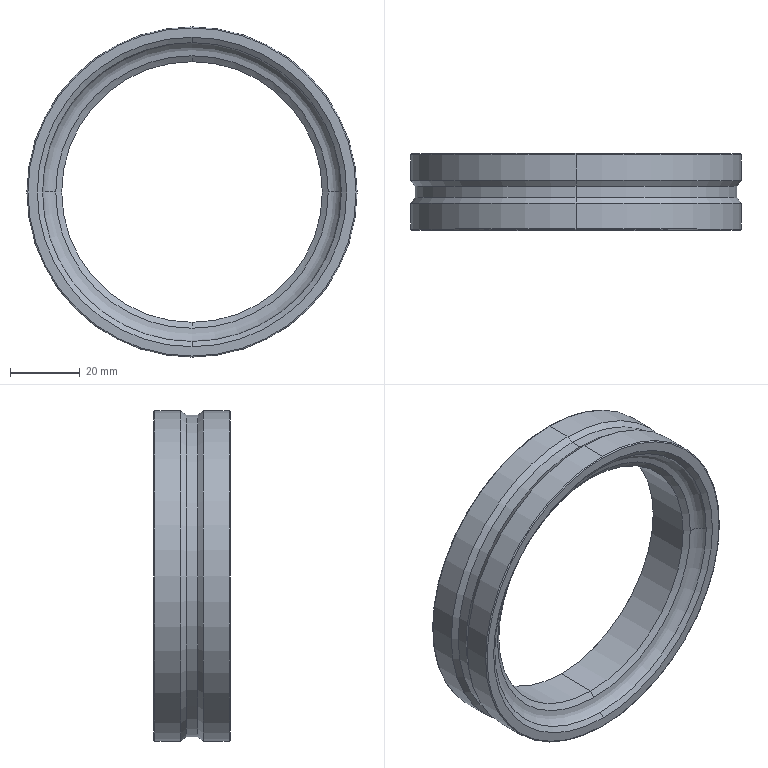Part | SolidWorks | features BaseBody 1 | 1 solid | 30 faces | box 95 x 22 x 95 mm | volume 47196 mm3 | cone 12 | torus 8 | cylinder 8 | plane 2 | commonest cylinder face diameters 95 x4 75 x2 92.6 x2
STEP:
#1=CARTESIAN_POINT('',(-2132.95,902.097,-1533.124));
#2=VERTEX_POINT('',#1);
#3=CARTESIAN_POINT('',(-2132.95,902.097,-1622.124));
#4=VERTEX_POINT('',#3);
#5=CARTESIAN_POINT('',(-2132.95,902.097,-1577.624));
#6=DIRECTION('',(0.,-1.,0.));
#7=DIRECTION('',(0.,0.,1.));
#8=AXIS2_PLACEMENT_3D('',#5,#6,#7);
#9=CIRCLE('',#8,44.5);
#10=EDGE_CURVE('',#2,#4,#9,.T.);
#11=ORIENTED_EDGE('',*,*,#10,.F.);
#12=CARTESIAN_POINT('',(-2132.95,902.097,-1577.624));
#13=DIRECTION('',(0.,-1.,0.));
#14=DIRECTION('',(0.,0.,-1.));
#15=AXIS2_PLACEMENT_3D('',#12,#13,#14);
#16=CIRCLE('',#15,44.5);
#17=EDGE_CURVE('',#4,#2,#16,.T.);
#18=ORIENTED_EDGE('',*,*,#17,.F.);
#19=EDGE_LOOP('',(#11,#18));
#20=FACE_BOUND('',#19,.T.);
#21=CARTESIAN_POINT('',(-2180.15,902.097,-1577.624));
#22=VERTEX_POINT('',#21);
#23=CARTESIAN_POINT('',(-2085.75,902.097,-1577.624));
#24=VERTEX_POINT('',#23);
#25=CARTESIAN_POINT('',(-2132.95,902.097,-1577.624));
#26=DIRECTION('',(0.,-1.,0.));
#27=DIRECTION('',(-1.,0.,0.));
#28=AXIS2_PLACEMENT_3D('',#25,#26,#27);
#29=CIRCLE('',#28,47.2);
#30=EDGE_CURVE('',#22,#24,#29,.T.);
#31=ORIENTED_EDGE('',*,*,#30,.T.);
#32=CARTESIAN_POINT('',(-2132.95,902.097,-1577.624));
#33=DIRECTION('',(0.,-1.,0.));
#34=DIRECTION('',(1.,0.,0.));
#35=AXIS2_PLACEMENT_3D('',#32,#33,#34);
#36=CIRCLE('',#35,47.2);
#37=EDGE_CURVE('',#24,#22,#36,.T.);
#38=ORIENTED_EDGE('',*,*,#37,.T.);
#39=EDGE_LOOP('',(#31,#38));
#40=FACE_OUTER_BOUND('',#39,.T.);
#41=CARTESIAN_POINT('',(-2081.03,902.097,-1629.544));
#42=DIRECTION('',(0.,-1.,0.));
#43=DIRECTION('',(0.,0.,-1.));
#44=AXIS2_PLACEMENT_3D('',#41,#42,#43);
#45=PLANE('',#44);
#46=ADVANCED_FACE('',(#20,#40),#45,.T.);
#47=CARTESIAN_POINT('',(-2132.95,903.147,-1620.624));
#48=VERTEX_POINT('',#47);
#49=CARTESIAN_POINT('',(-2132.95,902.097,-1622.124));
#50=DIRECTION('',(0.,0.5736,0.8192));
#51=VECTOR('',#50,1000.);
#52=LINE('',#49,#51);
#53=EDGE_CURVE('',#4,#48,#52,.T.);
#54=ORIENTED_EDGE('',*,*,#53,.T.);
#55=CARTESIAN_POINT('',(-2175.95,903.147,-1577.624));
#56=VERTEX_POINT('',#55);
#57=CARTESIAN_POINT('',(-2132.95,903.147,-1577.624));
#58=DIRECTION('',(0.,1.,0.));
#59=DIRECTION('',(0.,0.,-1.));
#60=AXIS2_PLACEMENT_3D('',#57,#58,#59);
#61=CIRCLE('',#60,43.);
#62=EDGE_CURVE('',#48,#56,#61,.T.);
#63=ORIENTED_EDGE('',*,*,#62,.T.);
#64=CARTESIAN_POINT('',(-2132.95,903.147,-1534.624));
#65=VERTEX_POINT('',#64);
#66=CARTESIAN_POINT('',(-2132.95,903.147,-1577.624));
#67=DIRECTION('',(0.,1.,0.));
#68=DIRECTION('',(-1.,0.,0.));
#69=AXIS2_PLACEMENT_3D('',#66,#67,#68);
#70=CIRCLE('',#69,43.);
#71=EDGE_CURVE('',#56,#65,#70,.T.);
#72=ORIENTED_EDGE('',*,*,#71,.T.);
#73=CARTESIAN_POINT('',(-2132.95,903.147,-1534.624));
#74=DIRECTION('',(0.,-0.5736,0.8192));
#75=VECTOR('',#74,1000.);
#76=LINE('',#73,#75);
#77=EDGE_CURVE('',#65,#2,#76,.T.);
#78=ORIENTED_EDGE('',*,*,#77,.T.);
#79=ORIENTED_EDGE('',*,*,#10,.T.);
#80=EDGE_LOOP('',(#54,#63,#72,#78,#79));
#81=FACE_OUTER_BOUND('',#80,.T.);
#82=CARTESIAN_POINT('',(-2132.95,903.2,-1577.624));
#83=DIRECTION('',(0.,-1.,0.));
#84=DIRECTION('',(0.08716,0.,-0.9962));
#85=AXIS2_PLACEMENT_3D('',#82,#83,#84);
#86=CONICAL_SURFACE('',#85,42.925,0.9599);
#87=ADVANCED_FACE('',(#81),#86,.F.);
#88=CARTESIAN_POINT('',(-2093.76,905.815,-1577.624));
#89=VERTEX_POINT('',#88);
#90=CARTESIAN_POINT('',(-2089.95,903.147,-1577.624));
#91=VERTEX_POINT('',#90);
#92=CARTESIAN_POINT('',(-2093.7,901.847,-1577.624));
#93=DIRECTION('',(0.,0.,-1.));
#94=DIRECTION('',(-0.01527,0.9999,0.));
#95=AXIS2_PLACEMENT_3D('',#92,#93,#94);
#96=CIRCLE('',#95,3.969);
#97=EDGE_CURVE('',#89,#91,#96,.T.);
#98=ORIENTED_EDGE('',*,*,#97,.T.);
#99=CARTESIAN_POINT('',(-2132.95,903.147,-1577.624));
#100=DIRECTION('',(0.,1.,0.));
#101=DIRECTION('',(0.,0.,1.));
#102=AXIS2_PLACEMENT_3D('',#99,#100,#101);
#103=CIRCLE('',#102,43.);
#104=EDGE_CURVE('',#65,#91,#103,.T.);
#105=ORIENTED_EDGE('',*,*,#104,.F.);
#106=ORIENTED_EDGE('',*,*,#71,.F.);
#107=CARTESIAN_POINT('',(-2172.139,905.815,-1577.624));
#108=VERTEX_POINT('',#107);
#109=CARTESIAN_POINT('',(-2172.2,901.847,-1577.624));
#110=DIRECTION('',(0.,0.,-1.));
#111=DIRECTION('',(-0.9448,0.3276,0.));
#112=AXIS2_PLACEMENT_3D('',#109,#110,#111);
#113=CIRCLE('',#112,3.969);
#114=EDGE_CURVE('',#56,#108,#113,.T.);
#115=ORIENTED_EDGE('',*,*,#114,.T.);
#116=CARTESIAN_POINT('',(-2132.95,905.815,-1538.435));
#117=VERTEX_POINT('',#116);
#118=CARTESIAN_POINT('',(-2132.95,905.815,-1577.624));
#119=DIRECTION('',(0.,1.,0.));
#120=DIRECTION('',(-1.,0.,0.));
#121=AXIS2_PLACEMENT_3D('',#118,#119,#120);
#122=CIRCLE('',#121,39.189);
#123=EDGE_CURVE('',#108,#117,#122,.T.);
#124=ORIENTED_EDGE('',*,*,#123,.T.);
#125=CARTESIAN_POINT('',(-2132.95,905.815,-1577.624));
#126=DIRECTION('',(0.,1.,0.));
#127=DIRECTION('',(0.,0.,1.));
#128=AXIS2_PLACEMENT_3D('',#125,#126,#127);
#129=CIRCLE('',#128,39.189);
#130=EDGE_CURVE('',#117,#89,#129,.T.);
#131=ORIENTED_EDGE('',*,*,#130,.T.);
#132=EDGE_LOOP('',(#98,#105,#106,#115,#124,#131));
#133=FACE_OUTER_BOUND('',#132,.T.);
#134=CARTESIAN_POINT('',(-2132.95,901.847,-1577.624));
#135=DIRECTION('',(0.,1.,0.));
#136=DIRECTION('',(-0.9962,0.,-0.08716));
#137=AXIS2_PLACEMENT_3D('',#134,#135,#136);
#138=TOROIDAL_SURFACE('',#137,39.25,3.969);
#139=ADVANCED_FACE('',(#133),#138,.F.);
#140=CARTESIAN_POINT('',(-2132.95,905.815,-1616.814));
#141=VERTEX_POINT('',#140);
#142=CARTESIAN_POINT('',(-2132.95,906.998,-1615.124));
#143=VERTEX_POINT('',#142);
#144=CARTESIAN_POINT('',(-2132.95,905.815,-1616.814));
#145=DIRECTION('',(0.,0.5736,0.8192));
#146=VECTOR('',#145,1000.);
#147=LINE('',#144,#146);
#148=EDGE_CURVE('',#141,#143,#147,.T.);
#149=ORIENTED_EDGE('',*,*,#148,.T.);
#150=CARTESIAN_POINT('',(-2132.95,906.998,-1540.124));
#151=VERTEX_POINT('',#150);
#152=CARTESIAN_POINT('',(-2132.95,906.998,-1577.624));
#153=DIRECTION('',(0.,1.,0.));
#154=DIRECTION('',(0.,0.,-1.));
#155=AXIS2_PLACEMENT_3D('',#152,#153,#154);
#156=CIRCLE('',#155,37.5);
#157=EDGE_CURVE('',#143,#151,#156,.T.);
#158=ORIENTED_EDGE('',*,*,#157,.T.);
#159=CARTESIAN_POINT('',(-2132.95,906.998,-1540.124));
#160=DIRECTION('',(0.,-0.5736,0.8192));
#161=VECTOR('',#160,1000.);
#162=LINE('',#159,#161);
#163=EDGE_CURVE('',#151,#117,#162,.T.);
#164=ORIENTED_EDGE('',*,*,#163,.T.);
#165=ORIENTED_EDGE('',*,*,#123,.F.);
#166=CARTESIAN_POINT('',(-2132.95,905.815,-1577.624));
#167=DIRECTION('',(0.,1.,0.));
#168=DIRECTION('',(0.,0.,-1.));
#169=AXIS2_PLACEMENT_3D('',#166,#167,#168);
#170=CIRCLE('',#169,39.189);
#171=EDGE_CURVE('',#141,#108,#170,.T.);
#172=ORIENTED_EDGE('',*,*,#171,.F.);
#173=EDGE_LOOP('',(#149,#158,#164,#165,#172));
#174=FACE_OUTER_BOUND('',#173,.T.);
#175=CARTESIAN_POINT('',(-2132.95,907.057,-1577.624));
#176=DIRECTION('',(0.,-1.,0.));
#177=DIRECTION('',(0.08716,0.,-0.9962));
#178=AXIS2_PLACEMENT_3D('',#175,#176,#177);
#179=CONICAL_SURFACE('',#178,37.416,0.9599);
#180=ADVANCED_FACE('',(#174),#179,.F.);
#181=CARTESIAN_POINT('',(-2132.95,919.195,-1615.124));
#182=VERTEX_POINT('',#181);
#183=CARTESIAN_POINT('',(-2132.95,906.998,-1615.124));
#184=DIRECTION('',(0.,1.,0.));
#185=VECTOR('',#184,1000.);
#186=LINE('',#183,#185);
#187=EDGE_CURVE('',#143,#182,#186,.T.);
#188=ORIENTED_EDGE('',*,*,#187,.T.);
#189=CARTESIAN_POINT('',(-2132.95,919.195,-1540.124));
#190=VERTEX_POINT('',#189);
#191=CARTESIAN_POINT('',(-2132.95,919.195,-1577.624));
#192=DIRECTION('',(0.,1.,0.));
#193=DIRECTION('',(0.,0.,-1.));
#194=AXIS2_PLACEMENT_3D('',#191,#192,#193);
#195=CIRCLE('',#194,37.5);
#196=EDGE_CURVE('',#182,#190,#195,.T.);
#197=ORIENTED_EDGE('',*,*,#196,.T.);
#198=CARTESIAN_POINT('',(-2132.95,919.195,-1540.124));
#199=DIRECTION('',(0.,-1.,0.));
#200=VECTOR('',#199,1000.);
#201=LINE('',#198,#200);
#202=EDGE_CURVE('',#190,#151,#201,.T.);
#203=ORIENTED_EDGE('',*,*,#202,.T.);
#204=ORIENTED_EDGE('',*,*,#157,.F.);
#205=EDGE_LOOP('',(#188,#197,#203,#204));
#206=FACE_OUTER_BOUND('',#205,.T.);
#207=CARTESIAN_POINT('',(-2132.95,919.805,-1577.624));
#208=DIRECTION('',(0.,-1.,0.));
#209=DIRECTION('',(0.08716,0.,0.9962));
#210=AXIS2_PLACEMENT_3D('',#207,#208,#209);
#211=CYLINDRICAL_SURFACE('',#210,37.5);
#212=ADVANCED_FACE('',(#206),#211,.F.);
#213=CARTESIAN_POINT('',(-2132.95,920.378,-1616.814));
#214=VERTEX_POINT('',#213);
#215=CARTESIAN_POINT('',(-2132.95,919.195,-1615.124));
#216=DIRECTION('',(0.,0.5736,-0.8192));
#217=VECTOR('',#216,1000.);
#218=LINE('',#215,#217);
#219=EDGE_CURVE('',#182,#214,#218,.T.);
#220=ORIENTED_EDGE('',*,*,#219,.T.);
#221=CARTESIAN_POINT('',(-2172.139,920.378,-1577.624));
#222=VERTEX_POINT('',#221);
#223=CARTESIAN_POINT('',(-2132.95,920.378,-1577.624));
#224=DIRECTION('',(0.,1.,0.));
#225=DIRECTION('',(0.,0.,-1.));
#226=AXIS2_PLACEMENT_3D('',#223,#224,#225);
#227=CIRCLE('',#226,39.189);
#228=EDGE_CURVE('',#214,#222,#227,.T.);
#229=ORIENTED_EDGE('',*,*,#228,.T.);
#230=CARTESIAN_POINT('',(-2132.95,920.378,-1538.435));
#231=VERTEX_POINT('',#230);
#232=CARTESIAN_POINT('',(-2132.95,920.378,-1577.624));
#233=DIRECTION('',(0.,1.,0.));
#234=DIRECTION('',(-1.,0.,0.));
#235=AXIS2_PLACEMENT_3D('',#232,#233,#234);
#236=CIRCLE('',#235,39.189);
#237=EDGE_CURVE('',#222,#231,#236,.T.);
#238=ORIENTED_EDGE('',*,*,#237,.T.);
#239=CARTESIAN_POINT('',(-2132.95,920.378,-1538.435));
#240=DIRECTION('',(0.,-0.5736,-0.8192));
#241=VECTOR('',#240,1000.);
#242=LINE('',#239,#241);
#243=EDGE_CURVE('',#231,#190,#242,.T.);
#244=ORIENTED_EDGE('',*,*,#243,.T.);
#245=ORIENTED_EDGE('',*,*,#196,.F.);
#246=EDGE_LOOP('',(#220,#229,#238,#244,#245));
#247=FACE_OUTER_BOUND('',#246,.T.);
#248=CARTESIAN_POINT('',(-2132.95,919.136,-1577.624));
#249=DIRECTION('',(0.,1.,0.));
#250=DIRECTION('',(0.08716,0.,0.9962));
#251=AXIS2_PLACEMENT_3D('',#248,#249,#250);
#252=CONICAL_SURFACE('',#251,37.416,0.9599);
#253=ADVANCED_FACE('',(#247),#252,.F.);
#254=CARTESIAN_POINT('',(-2089.95,923.046,-1577.624));
#255=VERTEX_POINT('',#254);
#256=CARTESIAN_POINT('',(-2093.76,920.378,-1577.624));
#257=VERTEX_POINT('',#256);
#258=CARTESIAN_POINT('',(-2093.7,924.347,-1577.624));
#259=DIRECTION('',(0.,0.,-1.));
#260=DIRECTION('',(0.9448,-0.3276,0.));
#261=AXIS2_PLACEMENT_3D('',#258,#259,#260);
#262=CIRCLE('',#261,3.969);
#263=EDGE_CURVE('',#255,#257,#262,.T.);
#264=ORIENTED_EDGE('',*,*,#263,.T.);
#265=CARTESIAN_POINT('',(-2132.95,920.378,-1577.624));
#266=DIRECTION('',(0.,1.,0.));
#267=DIRECTION('',(0.,0.,1.));
#268=AXIS2_PLACEMENT_3D('',#265,#266,#267);
#269=CIRCLE('',#268,39.189);
#270=EDGE_CURVE('',#231,#257,#269,.T.);
#271=ORIENTED_EDGE('',*,*,#270,.F.);
#272=ORIENTED_EDGE('',*,*,#237,.F.);
#273=CARTESIAN_POINT('',(-2175.95,923.046,-1577.624));
#274=VERTEX_POINT('',#273);
#275=CARTESIAN_POINT('',(-2172.2,924.347,-1577.624));
#276=DIRECTION('',(0.,0.,-1.));
#277=DIRECTION('',(0.01527,-0.9999,0.));
#278=AXIS2_PLACEMENT_3D('',#275,#276,#277);
#279=CIRCLE('',#278,3.969);
#280=EDGE_CURVE('',#222,#274,#279,.T.);
#281=ORIENTED_EDGE('',*,*,#280,.T.);
#282=CARTESIAN_POINT('',(-2132.95,923.046,-1534.624));
#283=VERTEX_POINT('',#282);
#284=CARTESIAN_POINT('',(-2132.95,923.046,-1577.624));
#285=DIRECTION('',(0.,1.,0.));
#286=DIRECTION('',(-1.,0.,0.));
#287=AXIS2_PLACEMENT_3D('',#284,#285,#286);
#288=CIRCLE('',#287,43.);
#289=EDGE_CURVE('',#274,#283,#288,.T.);
#290=ORIENTED_EDGE('',*,*,#289,.T.);
#291=CARTESIAN_POINT('',(-2132.95,923.046,-1577.624));
#292=DIRECTION('',(0.,1.,0.));
#293=DIRECTION('',(0.,0.,1.));
#294=AXIS2_PLACEMENT_3D('',#291,#292,#293);
#295=CIRCLE('',#294,43.);
#296=EDGE_CURVE('',#283,#255,#295,.T.);
#297=ORIENTED_EDGE('',*,*,#296,.T.);
#298=EDGE_LOOP('',(#264,#271,#272,#281,#290,#297));
#299=FACE_OUTER_BOUND('',#298,.T.);
#300=CARTESIAN_POINT('',(-2132.95,924.347,-1577.624));
#301=DIRECTION('',(0.,1.,0.));
#302=DIRECTION('',(-0.9962,0.,-0.08716));
#303=AXIS2_PLACEMENT_3D('',#300,#301,#302);
#304=TOROIDAL_SURFACE('',#303,39.25,3.969);
#305=ADVANCED_FACE('',(#299),#304,.F.);
#306=CARTESIAN_POINT('',(-2132.95,923.046,-1620.624));
#307=VERTEX_POINT('',#306);
#308=CARTESIAN_POINT('',(-2132.95,924.097,-1622.124));
#309=VERTEX_POINT('',#308);
#310=CARTESIAN_POINT('',(-2132.95,923.046,-1620.624));
#311=DIRECTION('',(0.,0.5736,-0.8192));
#312=VECTOR('',#311,1000.);
#313=LINE('',#310,#312);
#314=EDGE_CURVE('',#307,#309,#313,.T.);
#315=ORIENTED_EDGE('',*,*,#314,.T.);
#316=CARTESIAN_POINT('',(-2132.95,924.097,-1533.124));
#317=VERTEX_POINT('',#316);
#318=CARTESIAN_POINT('',(-2132.95,924.097,-1577.624));
#319=DIRECTION('',(0.,1.,0.));
#320=DIRECTION('',(0.,0.,-1.));
#321=AXIS2_PLACEMENT_3D('',#318,#319,#320);
#322=CIRCLE('',#321,44.5);
#323=EDGE_CURVE('',#309,#317,#322,.T.);
#324=ORIENTED_EDGE('',*,*,#323,.T.);
#325=CARTESIAN_POINT('',(-2132.95,924.097,-1533.124));
#326=DIRECTION('',(0.,-0.5736,-0.8192));
#327=VECTOR('',#326,1000.);
#328=LINE('',#325,#327);
#329=EDGE_CURVE('',#317,#283,#328,.T.);
#330=ORIENTED_EDGE('',*,*,#329,.T.);
#331=ORIENTED_EDGE('',*,*,#289,.F.);
#332=CARTESIAN_POINT('',(-2132.95,923.046,-1577.624));
#333=DIRECTION('',(0.,1.,0.));
#334=DIRECTION('',(0.,0.,-1.));
#335=AXIS2_PLACEMENT_3D('',#332,#333,#334);
#336=CIRCLE('',#335,43.);
#337=EDGE_CURVE('',#307,#274,#336,.T.);
#338=ORIENTED_EDGE('',*,*,#337,.F.);
#339=EDGE_LOOP('',(#315,#324,#330,#331,#338));
#340=FACE_OUTER_BOUND('',#339,.T.);
#341=CARTESIAN_POINT('',(-2132.95,922.994,-1577.624));
#342=DIRECTION('',(0.,1.,0.));
#343=DIRECTION('',(0.08716,0.,0.9962));
#344=AXIS2_PLACEMENT_3D('',#341,#342,#343);
#345=CONICAL_SURFACE('',#344,42.925,0.9599);
#346=ADVANCED_FACE('',(#340),#345,.F.);
#347=ORIENTED_EDGE('',*,*,#323,.F.);
#348=CARTESIAN_POINT('',(-2132.95,924.097,-1577.624));
#349=DIRECTION('',(0.,1.,0.));
#350=DIRECTION('',(0.,0.,1.));
#351=AXIS2_PLACEMENT_3D('',#348,#349,#350);
#352=CIRCLE('',#351,44.5);
#353=EDGE_CURVE('',#317,#309,#352,.T.);
#354=ORIENTED_EDGE('',*,*,#353,.F.);
#355=EDGE_LOOP('',(#347,#354));
#356=FACE_BOUND('',#355,.T.);
#357=CARTESIAN_POINT('',(-2085.75,924.097,-1577.624));
#358=VERTEX_POINT('',#357);
#359=CARTESIAN_POINT('',(-2180.15,924.097,-1577.624));
#360=VERTEX_POINT('',#359);
#361=CARTESIAN_POINT('',(-2132.95,924.097,-1577.624));
#362=DIRECTION('',(0.,1.,0.));
#363=DIRECTION('',(0.,0.,-1.));
#364=AXIS2_PLACEMENT_3D('',#361,#362,#363);
#365=CIRCLE('',#364,47.2);
#366=EDGE_CURVE('',#358,#360,#365,.T.);
#367=ORIENTED_EDGE('',*,*,#366,.T.);
#368=CARTESIAN_POINT('',(-2132.95,924.097,-1577.624));
#369=DIRECTION('',(0.,1.,0.));
#370=DIRECTION('',(-1.,0.,0.));
#371=AXIS2_PLACEMENT_3D('',#368,#369,#370);
#372=CIRCLE('',#371,47.2);
#373=EDGE_CURVE('',#360,#358,#372,.T.);
#374=ORIENTED_EDGE('',*,*,#373,.T.);
#375=EDGE_LOOP('',(#367,#374));
#376=FACE_OUTER_BOUND('',#375,.T.);
#377=CARTESIAN_POINT('',(-2081.03,924.097,-1525.704));
#378=DIRECTION('',(0.,1.,0.));
#379=DIRECTION('',(1.,0.,0.));
#380=AXIS2_PLACEMENT_3D('',#377,#378,#379);
#381=PLANE('',#380);
#382=ADVANCED_FACE('',(#356,#376),#381,.T.);
#383=CARTESIAN_POINT('',(-2180.45,923.797,-1577.624));
#384=VERTEX_POINT('',#383);
#385=CARTESIAN_POINT('',(-2180.15,923.797,-1577.624));
#386=DIRECTION('',(0.,0.,-1.));
#387=DIRECTION('',(-1.,0.,0.));
#388=AXIS2_PLACEMENT_3D('',#385,#386,#387);
#389=CIRCLE('',#388,0.3);
#390=EDGE_CURVE('',#384,#360,#389,.T.);
#391=ORIENTED_EDGE('',*,*,#390,.T.);
#392=ORIENTED_EDGE('',*,*,#366,.F.);
#393=CARTESIAN_POINT('',(-2085.45,923.797,-1577.624));
#394=VERTEX_POINT('',#393);
#395=CARTESIAN_POINT('',(-2085.75,923.797,-1577.624));
#396=DIRECTION('',(0.,0.,-1.));
#397=DIRECTION('',(0.,1.,0.));
#398=AXIS2_PLACEMENT_3D('',#395,#396,#397);
#399=CIRCLE('',#398,0.3);
#400=EDGE_CURVE('',#358,#394,#399,.T.);
#401=ORIENTED_EDGE('',*,*,#400,.T.);
#402=CARTESIAN_POINT('',(-2132.95,923.797,-1625.124));
#403=VERTEX_POINT('',#402);
#404=CARTESIAN_POINT('',(-2132.95,923.797,-1577.624));
#405=DIRECTION('',(0.,1.,0.));
#406=DIRECTION('',(1.,0.,0.));
#407=AXIS2_PLACEMENT_3D('',#404,#405,#406);
#408=CIRCLE('',#407,47.5);
#409=EDGE_CURVE('',#394,#403,#408,.T.);
#410=ORIENTED_EDGE('',*,*,#409,.T.);
#411=CARTESIAN_POINT('',(-2132.95,923.797,-1577.624));
#412=DIRECTION('',(0.,1.,0.));
#413=DIRECTION('',(0.,0.,-1.));
#414=AXIS2_PLACEMENT_3D('',#411,#412,#413);
#415=CIRCLE('',#414,47.5);
#416=EDGE_CURVE('',#403,#384,#415,.T.);
#417=ORIENTED_EDGE('',*,*,#416,.T.);
#418=EDGE_LOOP('',(#391,#392,#401,#410,#417));
#419=FACE_OUTER_BOUND('',#418,.T.);
#420=CARTESIAN_POINT('',(-2132.95,923.797,-1577.624));
#421=DIRECTION('',(0.,1.,0.));
#422=DIRECTION('',(0.9962,0.,0.08716));
#423=AXIS2_PLACEMENT_3D('',#420,#421,#422);
#424=TOROIDAL_SURFACE('',#423,47.2,0.3);
#425=ADVANCED_FACE('',(#419),#424,.T.);
#426=CARTESIAN_POINT('',(-2132.95,916.347,-1625.124));
#427=VERTEX_POINT('',#426);
#428=CARTESIAN_POINT('',(-2132.95,916.347,-1625.124));
#429=DIRECTION('',(0.,1.,0.));
#430=VECTOR('',#429,1000.);
#431=LINE('',#428,#430);
#432=EDGE_CURVE('',#427,#403,#431,.T.);
#433=ORIENTED_EDGE('',*,*,#432,.T.);
#434=ORIENTED_EDGE('',*,*,#409,.F.);
#435=CARTESIAN_POINT('',(-2132.95,923.797,-1530.124));
#436=VERTEX_POINT('',#435);
#437=CARTESIAN_POINT('',(-2132.95,923.797,-1577.624));
#438=DIRECTION('',(0.,1.,0.));
#439=DIRECTION('',(0.,0.,1.));
#440=AXIS2_PLACEMENT_3D('',#437,#438,#439);
#441=CIRCLE('',#440,47.5);
#442=EDGE_CURVE('',#436,#394,#441,.T.);
#443=ORIENTED_EDGE('',*,*,#442,.F.);
#444=CARTESIAN_POINT('',(-2132.95,916.347,-1530.124));
#445=VERTEX_POINT('',#444);
#446=CARTESIAN_POINT('',(-2132.95,923.797,-1530.124));
#447=DIRECTION('',(0.,-1.,0.));
#448=VECTOR('',#447,1000.);
#449=LINE('',#446,#448);
#450=EDGE_CURVE('',#436,#445,#449,.T.);
#451=ORIENTED_EDGE('',*,*,#450,.T.);
#452=CARTESIAN_POINT('',(-2132.95,916.347,-1577.624));
#453=DIRECTION('',(0.,1.,0.));
#454=DIRECTION('',(0.,0.,1.));
#455=AXIS2_PLACEMENT_3D('',#452,#453,#454);
#456=CIRCLE('',#455,47.5);
#457=EDGE_CURVE('',#445,#427,#456,.T.);
#458=ORIENTED_EDGE('',*,*,#457,.T.);
#459=EDGE_LOOP('',(#433,#434,#443,#451,#458));
#460=FACE_OUTER_BOUND('',#459,.T.);
#461=CARTESIAN_POINT('',(-2132.95,915.974,-1577.624));
#462=DIRECTION('',(0.,-1.,0.));
#463=DIRECTION('',(-0.08716,0.,-0.9962));
#464=AXIS2_PLACEMENT_3D('',#461,#462,#463);
#465=CYLINDRICAL_SURFACE('',#464,47.5);
#466=ADVANCED_FACE('',(#460),#465,.T.);
#467=CARTESIAN_POINT('',(-2132.95,914.697,-1623.924));
#468=VERTEX_POINT('',#467);
#469=CARTESIAN_POINT('',(-2132.95,914.697,-1623.924));
#470=DIRECTION('',(0.,0.8087,-0.5882));
#471=VECTOR('',#470,1000.);
#472=LINE('',#469,#471);
#473=EDGE_CURVE('',#468,#427,#472,.T.);
#474=ORIENTED_EDGE('',*,*,#473,.T.);
#475=ORIENTED_EDGE('',*,*,#457,.F.);
#476=CARTESIAN_POINT('',(-2132.95,914.697,-1531.324));
#477=VERTEX_POINT('',#476);
#478=CARTESIAN_POINT('',(-2132.95,916.347,-1530.124));
#479=DIRECTION('',(0.,-0.8087,-0.5882));
#480=VECTOR('',#479,1000.);
#481=LINE('',#478,#480);
#482=EDGE_CURVE('',#445,#477,#481,.T.);
#483=ORIENTED_EDGE('',*,*,#482,.T.);
#484=CARTESIAN_POINT('',(-2132.95,914.697,-1577.624));
#485=DIRECTION('',(0.,1.,0.));
#486=DIRECTION('',(0.,0.,1.));
#487=AXIS2_PLACEMENT_3D('',#484,#485,#486);
#488=CIRCLE('',#487,46.3);
#489=EDGE_CURVE('',#477,#468,#488,.T.);
#490=ORIENTED_EDGE('',*,*,#489,.T.);
#491=EDGE_LOOP('',(#474,#475,#483,#490));
#492=FACE_OUTER_BOUND('',#491,.T.);
#493=CARTESIAN_POINT('',(-2132.95,914.614,-1577.624));
#494=DIRECTION('',(0.,1.,0.));
#495=DIRECTION('',(-0.08716,0.,0.9962));
#496=AXIS2_PLACEMENT_3D('',#493,#494,#495);
#497=CONICAL_SURFACE('',#496,46.24,0.6288);
#498=ADVANCED_FACE('',(#492),#497,.T.);
#499=CARTESIAN_POINT('',(-2132.95,911.497,-1623.924));
#500=VERTEX_POINT('',#499);
#501=CARTESIAN_POINT('',(-2132.95,911.497,-1623.924));
#502=DIRECTION('',(0.,1.,0.));
#503=VECTOR('',#502,1000.);
#504=LINE('',#501,#503);
#505=EDGE_CURVE('',#500,#468,#504,.T.);
#506=ORIENTED_EDGE('',*,*,#505,.T.);
#507=ORIENTED_EDGE('',*,*,#489,.F.);
#508=CARTESIAN_POINT('',(-2132.95,911.497,-1531.324));
#509=VERTEX_POINT('',#508);
#510=CARTESIAN_POINT('',(-2132.95,914.697,-1531.324));
#511=DIRECTION('',(0.,-1.,0.));
#512=VECTOR('',#511,1000.);
#513=LINE('',#510,#512);
#514=EDGE_CURVE('',#477,#509,#513,.T.);
#515=ORIENTED_EDGE('',*,*,#514,.T.);
#516=CARTESIAN_POINT('',(-2132.95,911.497,-1577.624));
#517=DIRECTION('',(0.,1.,0.));
#518=DIRECTION('',(0.,0.,1.));
#519=AXIS2_PLACEMENT_3D('',#516,#517,#518);
#520=CIRCLE('',#519,46.3);
#521=EDGE_CURVE('',#509,#500,#520,.T.);
#522=ORIENTED_EDGE('',*,*,#521,.T.);
#523=EDGE_LOOP('',(#506,#507,#515,#522));
#524=FACE_OUTER_BOUND('',#523,.T.);
#525=CARTESIAN_POINT('',(-2132.95,911.337,-1577.624));
#526=DIRECTION('',(0.,-1.,0.));
#527=DIRECTION('',(-0.08716,0.,-0.9962));
#528=AXIS2_PLACEMENT_3D('',#525,#526,#527);
#529=CYLINDRICAL_SURFACE('',#528,46.3);
#530=ADVANCED_FACE('',(#524),#529,.T.);
#531=CARTESIAN_POINT('',(-2132.95,909.847,-1625.124));
#532=VERTEX_POINT('',#531);
#533=CARTESIAN_POINT('',(-2132.95,909.847,-1625.124));
#534=DIRECTION('',(0.,0.8087,0.5882));
#535=VECTOR('',#534,1000.);
#536=LINE('',#533,#535);
#537=EDGE_CURVE('',#532,#500,#536,.T.);
#538=ORIENTED_EDGE('',*,*,#537,.T.);
#539=ORIENTED_EDGE('',*,*,#521,.F.);
#540=CARTESIAN_POINT('',(-2132.95,909.847,-1530.124));
#541=VERTEX_POINT('',#540);
#542=CARTESIAN_POINT('',(-2132.95,911.497,-1531.324));
#543=DIRECTION('',(0.,-0.8087,0.5882));
#544=VECTOR('',#543,1000.);
#545=LINE('',#542,#544);
#546=EDGE_CURVE('',#509,#541,#545,.T.);
#547=ORIENTED_EDGE('',*,*,#546,.T.);
#548=CARTESIAN_POINT('',(-2132.95,909.847,-1577.624));
#549=DIRECTION('',(0.,1.,0.));
#550=DIRECTION('',(0.,0.,1.));
#551=AXIS2_PLACEMENT_3D('',#548,#549,#550);
#552=CIRCLE('',#551,47.5);
#553=EDGE_CURVE('',#541,#532,#552,.T.);
#554=ORIENTED_EDGE('',*,*,#553,.T.);
#555=EDGE_LOOP('',(#538,#539,#547,#554));
#556=FACE_OUTER_BOUND('',#555,.T.);
#557=CARTESIAN_POINT('',(-2132.95,911.579,-1577.624));
#558=DIRECTION('',(0.,-1.,0.));
#559=DIRECTION('',(-0.08716,0.,-0.9962));
#560=AXIS2_PLACEMENT_3D('',#557,#558,#559);
#561=CONICAL_SURFACE('',#560,46.24,0.6288);
#562=ADVANCED_FACE('',(#556),#561,.T.);
#563=CARTESIAN_POINT('',(-2132.95,902.397,-1625.124));
#564=VERTEX_POINT('',#563);
#565=CARTESIAN_POINT('',(-2132.95,902.397,-1625.124));
#566=DIRECTION('',(0.,1.,0.));
#567=VECTOR('',#566,1000.);
#568=LINE('',#565,#567);
#569=EDGE_CURVE('',#564,#532,#568,.T.);
#570=ORIENTED_EDGE('',*,*,#569,.T.);
#571=ORIENTED_EDGE('',*,*,#553,.F.);
#572=CARTESIAN_POINT('',(-2132.95,902.397,-1530.124));
#573=VERTEX_POINT('',#572);
#574=CARTESIAN_POINT('',(-2132.95,909.847,-1530.124));
#575=DIRECTION('',(0.,-1.,0.));
#576=VECTOR('',#575,1000.);
#577=LINE('',#574,#576);
#578=EDGE_CURVE('',#541,#573,#577,.T.);
#579=ORIENTED_EDGE('',*,*,#578,.T.);
#580=CARTESIAN_POINT('',(-2085.45,902.397,-1577.624));
#581=VERTEX_POINT('',#580);
#582=CARTESIAN_POINT('',(-2132.95,902.397,-1577.624));
#583=DIRECTION('',(0.,1.,0.));
#584=DIRECTION('',(0.,0.,1.));
#585=AXIS2_PLACEMENT_3D('',#582,#583,#584);
#586=CIRCLE('',#585,47.5);
#587=EDGE_CURVE('',#573,#581,#586,.T.);
#588=ORIENTED_EDGE('',*,*,#587,.T.);
#589=CARTESIAN_POINT('',(-2132.95,902.397,-1577.624));
#590=DIRECTION('',(0.,1.,0.));
#591=DIRECTION('',(1.,0.,0.));
#592=AXIS2_PLACEMENT_3D('',#589,#590,#591);
#593=CIRCLE('',#592,47.5);
#594=EDGE_CURVE('',#581,#564,#593,.T.);
#595=ORIENTED_EDGE('',*,*,#594,.T.);
#596=EDGE_LOOP('',(#570,#571,#579,#588,#595));
#597=FACE_OUTER_BOUND('',#596,.T.);
#598=CARTESIAN_POINT('',(-2132.95,902.024,-1577.624));
#599=DIRECTION('',(0.,-1.,0.));
#600=DIRECTION('',(-0.08716,0.,-0.9962));
#601=AXIS2_PLACEMENT_3D('',#598,#599,#600);
#602=CYLINDRICAL_SURFACE('',#601,47.5);
#603=ADVANCED_FACE('',(#597),#602,.T.);
#604=CARTESIAN_POINT('',(-2180.45,902.397,-1577.624));
#605=VERTEX_POINT('',#604);
#606=CARTESIAN_POINT('',(-2180.15,902.397,-1577.624));
#607=DIRECTION('',(0.,0.,-1.));
#608=DIRECTION('',(0.,-1.,0.));
#609=AXIS2_PLACEMENT_3D('',#606,#607,#608);
#610=CIRCLE('',#609,0.3);
#611=EDGE_CURVE('',#22,#605,#610,.T.);
#612=ORIENTED_EDGE('',*,*,#611,.T.);
#613=CARTESIAN_POINT('',(-2132.95,902.397,-1577.624));
#614=DIRECTION('',(0.,1.,0.));
#615=DIRECTION('',(0.,0.,-1.));
#616=AXIS2_PLACEMENT_3D('',#613,#614,#615);
#617=CIRCLE('',#616,47.5);
#618=EDGE_CURVE('',#564,#605,#617,.T.);
#619=ORIENTED_EDGE('',*,*,#618,.F.);
#620=ORIENTED_EDGE('',*,*,#594,.F.);
#621=CARTESIAN_POINT('',(-2085.75,902.397,-1577.624));
#622=DIRECTION('',(0.,0.,-1.));
#623=DIRECTION('',(1.,0.,0.));
#624=AXIS2_PLACEMENT_3D('',#621,#622,#623);
#625=CIRCLE('',#624,0.3);
#626=EDGE_CURVE('',#581,#24,#625,.T.);
#627=ORIENTED_EDGE('',*,*,#626,.T.);
#628=ORIENTED_EDGE('',*,*,#30,.F.);
#629=EDGE_LOOP('',(#612,#619,#620,#627,#628));
#630=FACE_OUTER_BOUND('',#629,.T.);
#631=CARTESIAN_POINT('',(-2132.95,902.397,-1577.624));
#632=DIRECTION('',(0.,1.,0.));
#633=DIRECTION('',(0.9962,0.,0.08716));
#634=AXIS2_PLACEMENT_3D('',#631,#632,#633);
#635=TOROIDAL_SURFACE('',#634,47.2,0.3);
#636=ADVANCED_FACE('',(#630),#635,.T.);
#637=ORIENTED_EDGE('',*,*,#611,.F.);
#638=ORIENTED_EDGE('',*,*,#37,.F.);
#639=ORIENTED_EDGE('',*,*,#626,.F.);
#640=ORIENTED_EDGE('',*,*,#587,.F.);
#641=CARTESIAN_POINT('',(-2132.95,902.397,-1577.624));
#642=DIRECTION('',(0.,1.,0.));
#643=DIRECTION('',(-1.,0.,0.));
#644=AXIS2_PLACEMENT_3D('',#641,#642,#643);
#645=CIRCLE('',#644,47.5);
#646=EDGE_CURVE('',#605,#573,#645,.T.);
#647=ORIENTED_EDGE('',*,*,#646,.F.);
#648=EDGE_LOOP('',(#637,#638,#639,#640,#647));
#649=FACE_OUTER_BOUND('',#648,.T.);
#650=CARTESIAN_POINT('',(-2132.95,902.397,-1577.624));
#651=DIRECTION('',(0.,1.,0.));
#652=DIRECTION('',(-0.9962,0.,-0.08716));
#653=AXIS2_PLACEMENT_3D('',#650,#651,#652);
#654=TOROIDAL_SURFACE('',#653,47.2,0.3);
#655=ADVANCED_FACE('',(#649),#654,.T.);
#656=ORIENTED_EDGE('',*,*,#569,.F.);
#657=ORIENTED_EDGE('',*,*,#618,.T.);
#658=ORIENTED_EDGE('',*,*,#646,.T.);
#659=ORIENTED_EDGE('',*,*,#578,.F.);
#660=CARTESIAN_POINT('',(-2132.95,909.847,-1577.624));
#661=DIRECTION('',(0.,1.,0.));
#662=DIRECTION('',(0.,0.,-1.));
#663=AXIS2_PLACEMENT_3D('',#660,#661,#662);
#664=CIRCLE('',#663,47.5);
#665=EDGE_CURVE('',#532,#541,#664,.T.);
#666=ORIENTED_EDGE('',*,*,#665,.F.);
#667=EDGE_LOOP('',(#656,#657,#658,#659,#666));
#668=FACE_OUTER_BOUND('',#667,.T.);
#669=CARTESIAN_POINT('',(-2132.95,902.024,-1577.624));
#670=DIRECTION('',(0.,-1.,0.));
#671=DIRECTION('',(0.08716,0.,0.9962));
#672=AXIS2_PLACEMENT_3D('',#669,#670,#671);
#673=CYLINDRICAL_SURFACE('',#672,47.5);
#674=ADVANCED_FACE('',(#668),#673,.T.);
#675=ORIENTED_EDGE('',*,*,#537,.F.);
#676=ORIENTED_EDGE('',*,*,#665,.T.);
#677=ORIENTED_EDGE('',*,*,#546,.F.);
#678=CARTESIAN_POINT('',(-2132.95,911.497,-1577.624));
#679=DIRECTION('',(0.,1.,0.));
#680=DIRECTION('',(0.,0.,-1.));
#681=AXIS2_PLACEMENT_3D('',#678,#679,#680);
#682=CIRCLE('',#681,46.3);
#683=EDGE_CURVE('',#500,#509,#682,.T.);
#684=ORIENTED_EDGE('',*,*,#683,.F.);
#685=EDGE_LOOP('',(#675,#676,#677,#684));
#686=FACE_OUTER_BOUND('',#685,.T.);
#687=CARTESIAN_POINT('',(-2132.95,911.579,-1577.624));
#688=DIRECTION('',(0.,-1.,0.));
#689=DIRECTION('',(0.08716,0.,0.9962));
#690=AXIS2_PLACEMENT_3D('',#687,#688,#689);
#691=CONICAL_SURFACE('',#690,46.24,0.6288);
#692=ADVANCED_FACE('',(#686),#691,.T.);
#693=ORIENTED_EDGE('',*,*,#505,.F.);
#694=ORIENTED_EDGE('',*,*,#683,.T.);
#695=ORIENTED_EDGE('',*,*,#514,.F.);
#696=CARTESIAN_POINT('',(-2132.95,914.697,-1577.624));
#697=DIRECTION('',(0.,1.,0.));
#698=DIRECTION('',(0.,0.,-1.));
#699=AXIS2_PLACEMENT_3D('',#696,#697,#698);
#700=CIRCLE('',#699,46.3);
#701=EDGE_CURVE('',#468,#477,#700,.T.);
#702=ORIENTED_EDGE('',*,*,#701,.F.);
#703=EDGE_LOOP('',(#693,#694,#695,#702));
#704=FACE_OUTER_BOUND('',#703,.T.);
#705=CARTESIAN_POINT('',(-2132.95,911.337,-1577.624));
#706=DIRECTION('',(0.,-1.,0.));
#707=DIRECTION('',(0.08716,0.,0.9962));
#708=AXIS2_PLACEMENT_3D('',#705,#706,#707);
#709=CYLINDRICAL_SURFACE('',#708,46.3);
#710=ADVANCED_FACE('',(#704),#709,.T.);
#711=ORIENTED_EDGE('',*,*,#473,.F.);
#712=ORIENTED_EDGE('',*,*,#701,.T.);
#713=ORIENTED_EDGE('',*,*,#482,.F.);
#714=CARTESIAN_POINT('',(-2132.95,916.347,-1577.624));
#715=DIRECTION('',(0.,1.,0.));
#716=DIRECTION('',(0.,0.,-1.));
#717=AXIS2_PLACEMENT_3D('',#714,#715,#716);
#718=CIRCLE('',#717,47.5);
#719=EDGE_CURVE('',#427,#445,#718,.T.);
#720=ORIENTED_EDGE('',*,*,#719,.F.);
#721=EDGE_LOOP('',(#711,#712,#713,#720));
#722=FACE_OUTER_BOUND('',#721,.T.);
#723=CARTESIAN_POINT('',(-2132.95,914.614,-1577.624));
#724=DIRECTION('',(0.,1.,0.));
#725=DIRECTION('',(0.08716,0.,-0.9962));
#726=AXIS2_PLACEMENT_3D('',#723,#724,#725);
#727=CONICAL_SURFACE('',#726,46.24,0.6288);
#728=ADVANCED_FACE('',(#722),#727,.T.);
#729=ORIENTED_EDGE('',*,*,#432,.F.);
#730=ORIENTED_EDGE('',*,*,#719,.T.);
#731=ORIENTED_EDGE('',*,*,#450,.F.);
#732=CARTESIAN_POINT('',(-2132.95,923.797,-1577.624));
#733=DIRECTION('',(0.,1.,0.));
#734=DIRECTION('',(-1.,0.,0.));
#735=AXIS2_PLACEMENT_3D('',#732,#733,#734);
#736=CIRCLE('',#735,47.5);
#737=EDGE_CURVE('',#384,#436,#736,.T.);
#738=ORIENTED_EDGE('',*,*,#737,.F.);
#739=ORIENTED_EDGE('',*,*,#416,.F.);
#740=EDGE_LOOP('',(#729,#730,#731,#738,#739));
#741=FACE_OUTER_BOUND('',#740,.T.);
#742=CARTESIAN_POINT('',(-2132.95,915.974,-1577.624));
#743=DIRECTION('',(0.,-1.,0.));
#744=DIRECTION('',(0.08716,0.,0.9962));
#745=AXIS2_PLACEMENT_3D('',#742,#743,#744);
#746=CYLINDRICAL_SURFACE('',#745,47.5);
#747=ADVANCED_FACE('',(#741),#746,.T.);
#748=ORIENTED_EDGE('',*,*,#390,.F.);
#749=ORIENTED_EDGE('',*,*,#737,.T.);
#750=ORIENTED_EDGE('',*,*,#442,.T.);
#751=ORIENTED_EDGE('',*,*,#400,.F.);
#752=ORIENTED_EDGE('',*,*,#373,.F.);
#753=EDGE_LOOP('',(#748,#749,#750,#751,#752));
#754=FACE_OUTER_BOUND('',#753,.T.);
#755=CARTESIAN_POINT('',(-2132.95,923.797,-1577.624));
#756=DIRECTION('',(0.,1.,0.));
#757=DIRECTION('',(-0.9962,0.,-0.08716));
#758=AXIS2_PLACEMENT_3D('',#755,#756,#757);
#759=TOROIDAL_SURFACE('',#758,47.2,0.3);
#760=ADVANCED_FACE('',(#754),#759,.T.);
#761=ORIENTED_EDGE('',*,*,#314,.F.);
#762=CARTESIAN_POINT('',(-2132.95,923.046,-1577.624));
#763=DIRECTION('',(0.,1.,0.));
#764=DIRECTION('',(1.,0.,0.));
#765=AXIS2_PLACEMENT_3D('',#762,#763,#764);
#766=CIRCLE('',#765,43.);
#767=EDGE_CURVE('',#255,#307,#766,.T.);
#768=ORIENTED_EDGE('',*,*,#767,.F.);
#769=ORIENTED_EDGE('',*,*,#296,.F.);
#770=ORIENTED_EDGE('',*,*,#329,.F.);
#771=ORIENTED_EDGE('',*,*,#353,.T.);
#772=EDGE_LOOP('',(#761,#768,#769,#770,#771));
#773=FACE_OUTER_BOUND('',#772,.T.);
#774=CARTESIAN_POINT('',(-2132.95,922.994,-1577.624));
#775=DIRECTION('',(0.,1.,0.));
#776=DIRECTION('',(-0.08716,0.,-0.9962));
#777=AXIS2_PLACEMENT_3D('',#774,#775,#776);
#778=CONICAL_SURFACE('',#777,42.925,0.9599);
#779=ADVANCED_FACE('',(#773),#778,.F.);
#780=ORIENTED_EDGE('',*,*,#263,.F.);
#781=ORIENTED_EDGE('',*,*,#767,.T.);
#782=ORIENTED_EDGE('',*,*,#337,.T.);
#783=ORIENTED_EDGE('',*,*,#280,.F.);
#784=ORIENTED_EDGE('',*,*,#228,.F.);
#785=CARTESIAN_POINT('',(-2132.95,920.378,-1577.624));
#786=DIRECTION('',(0.,1.,0.));
#787=DIRECTION('',(1.,0.,0.));
#788=AXIS2_PLACEMENT_3D('',#785,#786,#787);
#789=CIRCLE('',#788,39.189);
#790=EDGE_CURVE('',#257,#214,#789,.T.);
#791=ORIENTED_EDGE('',*,*,#790,.F.);
#792=EDGE_LOOP('',(#780,#781,#782,#783,#784,#791));
#793=FACE_OUTER_BOUND('',#792,.T.);
#794=CARTESIAN_POINT('',(-2132.95,924.347,-1577.624));
#795=DIRECTION('',(0.,1.,0.));
#796=DIRECTION('',(0.9962,0.,0.08716));
#797=AXIS2_PLACEMENT_3D('',#794,#795,#796);
#798=TOROIDAL_SURFACE('',#797,39.25,3.969);
#799=ADVANCED_FACE('',(#793),#798,.F.);
#800=ORIENTED_EDGE('',*,*,#219,.F.);
#801=CARTESIAN_POINT('',(-2132.95,919.195,-1577.624));
#802=DIRECTION('',(0.,1.,0.));
#803=DIRECTION('',(0.,0.,1.));
#804=AXIS2_PLACEMENT_3D('',#801,#802,#803);
#805=CIRCLE('',#804,37.5);
#806=EDGE_CURVE('',#190,#182,#805,.T.);
#807=ORIENTED_EDGE('',*,*,#806,.F.);
#808=ORIENTED_EDGE('',*,*,#243,.F.);
#809=ORIENTED_EDGE('',*,*,#270,.T.);
#810=ORIENTED_EDGE('',*,*,#790,.T.);
#811=EDGE_LOOP('',(#800,#807,#808,#809,#810));
#812=FACE_OUTER_BOUND('',#811,.T.);
#813=CARTESIAN_POINT('',(-2132.95,919.136,-1577.624));
#814=DIRECTION('',(0.,1.,0.));
#815=DIRECTION('',(-0.08716,0.,-0.9962));
#816=AXIS2_PLACEMENT_3D('',#813,#814,#815);
#817=CONICAL_SURFACE('',#816,37.416,0.9599);
#818=ADVANCED_FACE('',(#812),#817,.F.);
#819=ORIENTED_EDGE('',*,*,#187,.F.);
#820=CARTESIAN_POINT('',(-2132.95,906.998,-1577.624));
#821=DIRECTION('',(0.,1.,0.));
#822=DIRECTION('',(0.,0.,1.));
#823=AXIS2_PLACEMENT_3D('',#820,#821,#822);
#824=CIRCLE('',#823,37.5);
#825=EDGE_CURVE('',#151,#143,#824,.T.);
#826=ORIENTED_EDGE('',*,*,#825,.F.);
#827=ORIENTED_EDGE('',*,*,#202,.F.);
#828=ORIENTED_EDGE('',*,*,#806,.T.);
#829=EDGE_LOOP('',(#819,#826,#827,#828));
#830=FACE_OUTER_BOUND('',#829,.T.);
#831=CARTESIAN_POINT('',(-2132.95,919.805,-1577.624));
#832=DIRECTION('',(0.,-1.,0.));
#833=DIRECTION('',(-0.08716,0.,-0.9962));
#834=AXIS2_PLACEMENT_3D('',#831,#832,#833);
#835=CYLINDRICAL_SURFACE('',#834,37.5);
#836=ADVANCED_FACE('',(#830),#835,.F.);
#837=ORIENTED_EDGE('',*,*,#148,.F.);
#838=CARTESIAN_POINT('',(-2132.95,905.815,-1577.624));
#839=DIRECTION('',(0.,1.,0.));
#840=DIRECTION('',(1.,0.,0.));
#841=AXIS2_PLACEMENT_3D('',#838,#839,#840);
#842=CIRCLE('',#841,39.189);
#843=EDGE_CURVE('',#89,#141,#842,.T.);
#844=ORIENTED_EDGE('',*,*,#843,.F.);
#845=ORIENTED_EDGE('',*,*,#130,.F.);
#846=ORIENTED_EDGE('',*,*,#163,.F.);
#847=ORIENTED_EDGE('',*,*,#825,.T.);
#848=EDGE_LOOP('',(#837,#844,#845,#846,#847));
#849=FACE_OUTER_BOUND('',#848,.T.);
#850=CARTESIAN_POINT('',(-2132.95,907.057,-1577.624));
#851=DIRECTION('',(0.,-1.,0.));
#852=DIRECTION('',(-0.08716,0.,0.9962));
#853=AXIS2_PLACEMENT_3D('',#850,#851,#852);
#854=CONICAL_SURFACE('',#853,37.416,0.9599);
#855=ADVANCED_FACE('',(#849),#854,.F.);
#856=ORIENTED_EDGE('',*,*,#97,.F.);
#857=ORIENTED_EDGE('',*,*,#843,.T.);
#858=ORIENTED_EDGE('',*,*,#171,.T.);
#859=ORIENTED_EDGE('',*,*,#114,.F.);
#860=ORIENTED_EDGE('',*,*,#62,.F.);
#861=CARTESIAN_POINT('',(-2132.95,903.147,-1577.624));
#862=DIRECTION('',(0.,1.,0.));
#863=DIRECTION('',(1.,0.,0.));
#864=AXIS2_PLACEMENT_3D('',#861,#862,#863);
#865=CIRCLE('',#864,43.);
#866=EDGE_CURVE('',#91,#48,#865,.T.);
#867=ORIENTED_EDGE('',*,*,#866,.F.);
#868=EDGE_LOOP('',(#856,#857,#858,#859,#860,#867));
#869=FACE_OUTER_BOUND('',#868,.T.);
#870=CARTESIAN_POINT('',(-2132.95,901.847,-1577.624));
#871=DIRECTION('',(0.,1.,0.));
#872=DIRECTION('',(0.9962,0.,0.08716));
#873=AXIS2_PLACEMENT_3D('',#870,#871,#872);
#874=TOROIDAL_SURFACE('',#873,39.25,3.969);
#875=ADVANCED_FACE('',(#869),#874,.F.);
#876=ORIENTED_EDGE('',*,*,#53,.F.);
#877=ORIENTED_EDGE('',*,*,#17,.T.);
#878=ORIENTED_EDGE('',*,*,#77,.F.);
#879=ORIENTED_EDGE('',*,*,#104,.T.);
#880=ORIENTED_EDGE('',*,*,#866,.T.);
#881=EDGE_LOOP('',(#876,#877,#878,#879,#880));
#882=FACE_OUTER_BOUND('',#881,.T.);
#883=CARTESIAN_POINT('',(-2132.95,903.2,-1577.624));
#884=DIRECTION('',(0.,-1.,0.));
#885=DIRECTION('',(-0.08716,0.,0.9962));
#886=AXIS2_PLACEMENT_3D('',#883,#884,#885);
#887=CONICAL_SURFACE('',#886,42.925,0.9599);
#888=ADVANCED_FACE('',(#882),#887,.F.);
#889=CLOSED_SHELL('',(#46,#87,#139,#180,#212,#253,#305,#346,#382,#425,#466,#498,#530,#562,#603,#636,#655,#674,#692,#710,#728,#747,#760,#779,#799,#818,#836,#855,#875,#888));
#890=MANIFOLD_SOLID_BREP('',#889);
#891=CARTESIAN_POINT('',(0.,0.,0.));
#892=DIRECTION('',(0.,0.,1.));
#893=DIRECTION('',(1.,0.,0.));
#894=AXIS2_PLACEMENT_3D('',#891,#892,#893);
#895=(LENGTH_UNIT()NAMED_UNIT(*)SI_UNIT(.MILLI.,.METRE.));
#896=UNCERTAINTY_MEASURE_WITH_UNIT(LENGTH_MEASURE(0.00001),#895,'','');
#897=(NAMED_UNIT(*)PLANE_ANGLE_UNIT()SI_UNIT($,.RADIAN.));
#898=(NAMED_UNIT(*)SI_UNIT($,.STERADIAN.)SOLID_ANGLE_UNIT());
#899=(GEOMETRIC_REPRESENTATION_CONTEXT(3)GLOBAL_UNCERTAINTY_ASSIGNED_CONTEXT((#896))GLOBAL_UNIT_ASSIGNED_CONTEXT((#895,#897,#898))REPRESENTATION_CONTEXT('',''));
#900=ADVANCED_BREP_SHAPE_REPRESENTATION('',(#890,#894),#899);